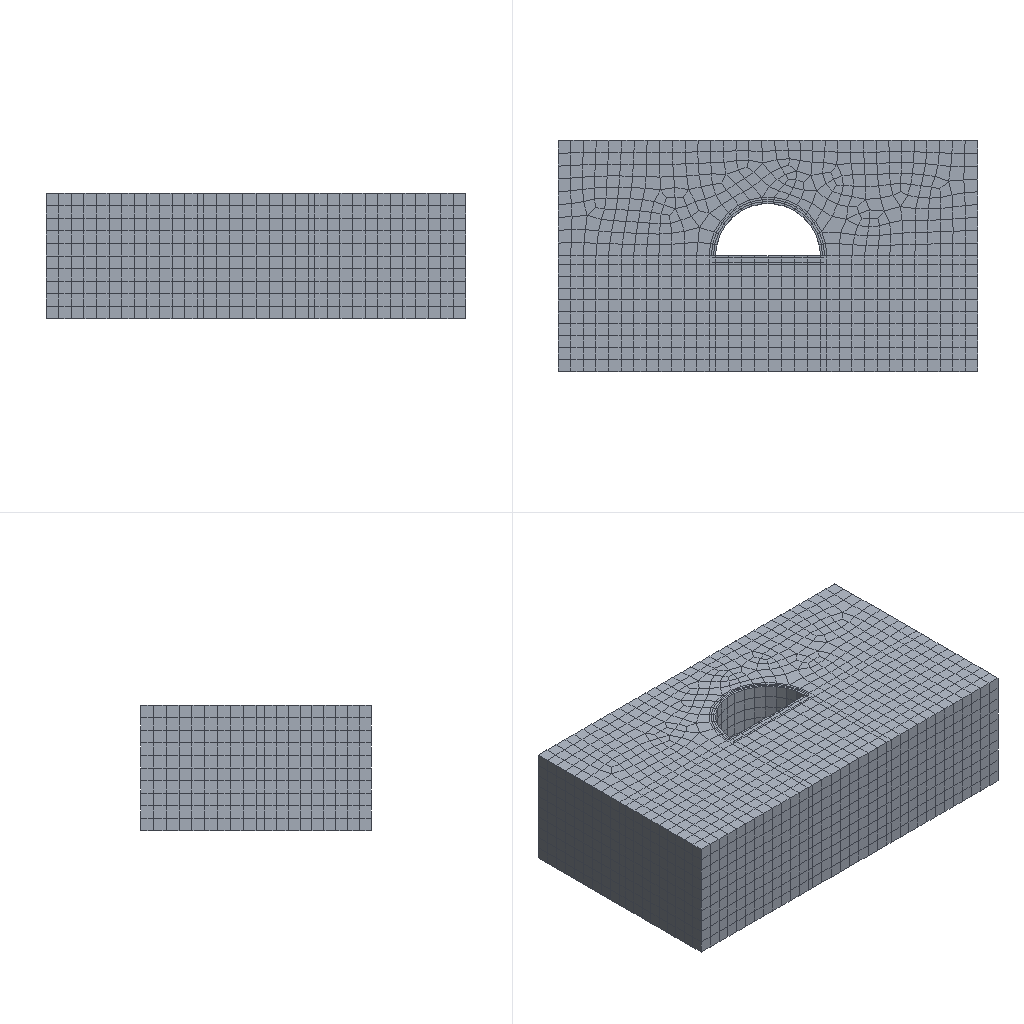Simulation study | abaqus
Set-up summary:
category,name,step,type,value,unit,region
solver,abaqus
solver,version,,,Abaqus/Standard 2020
units,not stated in the deck,,not stated
analysis,deck,,static,static
load_step,Step-1,Step-1,static
load_step,requested,,,1
mesh,nodes,,,8613
mesh,elements,,,7150
element_type,S4R,,shell,460
element_type,C3D8,,solid,6690
load,load commands in deck,,count,2
bc,support commands in deck,,count,7
material,CONCRETE,,in results
material,REBAR,,in results
material,SOIL,,in results
check,setup vs results,,match,"per instance, exact: element labels, types and connectivity; labels of the nodes the elements use; coordinates of those nodes at SINGLE_PRECISION in 5 of 5 instance(s)"
Abaqus input file, long lists of numbers shortened:
*Heading
** Job name: Job-1 Model name: Model-1
** Generated by: Abaqus/CAE 2020
*Preprint, echo=NO, model=NO, history=NO, contact=NO
**
** PARTS
**
*Part, name=Part-1
*Node
      1,  -2.8,   1.1,           6.
      2,  -2.8,   1.1,           0.
** (8061 more lines like these left out)
*Element, type=C3D8
  1,  98, 643, 742,  77,   1,  41,  58,   4
  2, 643, 644, 743, 742,  41,  42,  57,  58
** (6688 more lines like these left out)
*Nset, nset=Set-1
    1,    2,    3,    4,    5,    6,    7,    8,    9,   10,   13,   14,   15,   16,   17,   18
   19,   20,   21,   22,   25,   26,   27,   28,   29,   30,   31,   32,   33,   34,   35,   36
** (487 more lines like these left out)
*Elset, elset=Set-1
    1,    2,    3,    4,    5,    6,    7,    8,    9,   10,   11,   12,   13,   14,   15,   16
   17,   18,   19,   20,   21,   22,   23,   24,   25,   26,   27,   28,   29,   30,   31,   32
** (401 more lines like these left out)
*Nset, nset=Set-2
    1,    2,    3,    4,    9,   10,   11,   12,   20,   21,   23,   24,   25,   26,   27,   28
   41,   42,   43,   44,   45,   46,   47,   48,   49,   50,   51,   52,   53,   54,   55,   56
** (33 more lines like these left out)
*Elset, elset=Set-2
  121,  122,  123,  124,  125,  126,  127,  128,  129,  130, 2021, 2022, 2023, 2024, 2025, 2026
 2027, 2028, 2029, 2030, 2031, 2032, 2033, 2034, 2035, 2036, 2037, 2038, 2039, 2040, 2041, 2042
** (14 more lines like these left out)
*Nset, nset=Set-3
    1,    2,    3,    4,    9,   10,   11,   12,   20,   21,   23,   24,   25,   26,   27,   28
   41,   42,   43,   44,   45,   46,   47,   48,   49,   50,   51,   52,   53,   54,   55,   56
** (33 more lines like these left out)
*Elset, elset=Set-3
  121,  122,  123,  124,  125,  126,  127,  128,  129,  130, 2021, 2022, 2023, 2024, 2025, 2026
 2027, 2028, 2029, 2030, 2031, 2032, 2033, 2034, 2035, 2036, 2037, 2038, 2039, 2040, 2041, 2042
** (14 more lines like these left out)
*Nset, nset=Set-6
    1,    2,    3,    4,    5,    6,    7,    8,    9,   10,   13,   14,   15,   16,   17,   18
   19,   20,   21,   22,   25,   26,   27,   28,   29,   30,   31,   32,   33,   34,   35,   36
** (487 more lines like these left out)
*Elset, elset=Set-6
    1,    2,    3,    4,    5,    6,    7,    8,    9,   10,   11,   12,   13,   14,   15,   16
   17,   18,   19,   20,   21,   22,   23,   24,   25,   26,   27,   28,   29,   30,   31,   32
** (401 more lines like these left out)
*Nset, nset=Set-7
    1,    2,    3,    4,    9,   10,   11,   12,   20,   21,   23,   24,   25,   26,   27,   28
   41,   42,   43,   44,   45,   46,   47,   48,   49,   50,   51,   52,   53,   54,   55,   56
** (33 more lines like these left out)
*Elset, elset=Set-7
  121,  122,  123,  124,  125,  126,  127,  128,  129,  130, 2021, 2022, 2023, 2024, 2025, 2026
 2027, 2028, 2029, 2030, 2031, 2032, 2033, 2034, 2035, 2036, 2037, 2038, 2039, 2040, 2041, 2042
** (14 more lines like these left out)
*Nset, nset=Set-8
    1,    2,    3,    4,    5,    6,    7,    8,    9,   10,   13,   14,   15,   16,   17,   18
   19,   20,   21,   22,   25,   26,   27,   28,   29,   30,   31,   32,   33,   34,   35,   36
** (487 more lines like these left out)
*Elset, elset=Set-8
    1,    2,    3,    4,    5,    6,    7,    8,    9,   10,   11,   12,   13,   14,   15,   16
   17,   18,   19,   20,   21,   22,   23,   24,   25,   26,   27,   28,   29,   30,   31,   32
** (401 more lines like these left out)
*Nset, nset=Set-9
    1,    2,    3,    4,    9,   10,   11,   12,   20,   21,   23,   24,   25,   26,   27,   28
   41,   42,   43,   44,   45,   46,   47,   48,   49,   50,   51,   52,   53,   54,   55,   56
** (33 more lines like these left out)
*Elset, elset=Set-9
  121,  122,  123,  124,  125,  126,  127,  128,  129,  130, 2021, 2022, 2023, 2024, 2025, 2026
 2027, 2028, 2029, 2030, 2031, 2032, 2033, 2034, 2035, 2036, 2037, 2038, 2039, 2040, 2041, 2042
** (14 more lines like these left out)
** Section: Section-1-soil
*Solid Section, elset=Set-8, material=soil
,
** Section: Section-2-concrete
*Solid Section, elset=Set-9, material=concrete
,
*End Part
**
*Part, name=rebar-face
*Node
      1,   5.3,           0.,           0.
      2,   4.711,           0.,           0.
** (108 more lines like these left out)
*Element, type=S4R
 1,   1,   2,  12,  11
 2,   2,   3,  13,  12
** (88 more lines like these left out)
*Nset, nset=Set-1, generate
   1,  110,    1
*Elset, elset=Set-1, generate
  1,  90,   1
** Section: rebar
*Shell Section, elset=Set-1, material=rebar
0.001, 5
*End Part
**
*Part, name=rebar2point6
*Node
      1,    2.6,           0.,           6.
      2,   2.535,  0.5786,           6.
** (163 more lines like these left out)
*Element, type=S4R
  1,   1,   2,  17,  16
  2,   2,   3,  18,  17
** (138 more lines like these left out)
*Nset, nset=Set-1, generate
   1,  165,    1
*Elset, elset=Set-1, generate
   1,  140,    1
** Section: rebar
*Shell Section, elset=Set-1, material=rebar
0.001, 5
*End Part
**
*Part, name=rebar2point7
*Node
      1,   2.7,           0.,           6.
      2,   2.632,  0.6008,           6.
** (163 more lines like these left out)
*Element, type=S4R
  1,   1,   2,  17,  16
  2,   2,   3,  18,  17
** (138 more lines like these left out)
*Nset, nset=Set-1, generate
   1,  165,    1
*Elset, elset=Set-1, generate
   1,  140,    1
** Section: rebar
*Shell Section, elset=Set-1, material=rebar
0.001, 5
*End Part
**
**
** ASSEMBLY
**
*Assembly, name=Assembly
**
*Instance, name=Part-1-1, part=Part-1
*End Instance
**
*Instance, name=rebar2point6-1, part=rebar2point6
          0.,          1.5,           0.
*End Instance
**
*Instance, name=rebar2point7-1, part=rebar2point7
          0.,          1.5,           0.
*End Instance
**
*Instance, name=rebar-face-1, part=rebar-face
       -2.65,          1.4,           6.
       -2.65,          1.4,           6., -1.65,          1.4,           6., 90.
*End Instance
**
*Instance, name=rebar-face-1-lin-1-2, part=rebar-face
       -2.65,          1.2,           6.
       -2.65,          1.2,           6., -1.65,          1.2,           6., 90.
*End Instance
**
*Nset, nset=Set-1, instance=Part-1-1
    1,    4,    7,    8,    9,   12,   13,   14,   18,   21,   22,   23,   25,   28,   29,   31
   32,   36,   39,   40,   77,   78,   79,   80,   81,   82,   83,   84,   85,   86,   87,   88
** (44 more lines like these left out)
*Elset, elset=Set-1, instance=Part-1-1
    1,   11,   21,   31,   41,   51,   61,   71,   81,   91,  101,  111,  121,  131,  132,  133
  134,  135,  136,  137,  138,  139,  140,  141,  142,  143,  144,  145,  146,  147,  148,  149
** (40 more lines like these left out)
*Nset, nset=Set-2, instance=Part-1-1
    2,    3,    5,    6,   10,   11,   15,   16,   17,   19,   20,   24,   26,   27,   30,   33
   34,   35,   37,   38,   99,  100,  101,  102,  103,  104,  105,  106,  107,  108,  109,  110
** (44 more lines like these left out)
*Elset, elset=Set-2, instance=Part-1-1
   10,   20,   30,   40,   50,   60,   70,   80,   90,  100,  110,  120,  130, 1103, 1104, 1105
 1106, 1107, 1108, 1109, 1110, 1111, 1112, 1113, 1114, 1115, 1116, 1117, 1118, 1119, 1120, 1121
** (40 more lines like these left out)
*Nset, nset=Set-3, instance=Part-1-1
   31,   32,   33,   34,   35,   36,   38,   39,  364,  365,  366,  367,  368,  369,  370,  371
  372,  373,  374,  375,  376,  377,  378,  379,  380,  381,  382,  383,  384,  385,  386,  387
** (12 more lines like these left out)
*Elset, elset=Set-3, instance=Part-1-1
 3191, 3192, 3193, 3194, 3195, 3196, 3197, 3198, 3199, 3200, 3201, 3202, 3203, 3204, 3205, 3206
 3207, 3208, 3209, 3210, 3211, 3212, 3213, 3214, 3215, 3216, 3217, 3218, 3219, 3220, 3221, 3222
** (10 more lines like these left out)
*Nset, nset=Set-4, instance=Part-1-1
    5,    6,    7,    8,   14,   15,   37,   40,   59,   60,   61,   62,   63,   64,   65,   66
   67,   68,   69,   70,   71,   72,   73,   74,   75,   76,  147,  148,  149,  150,  151,  152
** (12 more lines like these left out)
*Elset, elset=Set-4, instance=Part-1-1
  111,  112,  113,  114,  115,  116,  117,  118,  119,  120,  230,  231,  232,  233,  234,  235
  236,  237,  238,  338,  339,  340,  341,  342,  343,  344,  345,  346,  446,  447,  448,  449
** (10 more lines like these left out)
*Nset, nset=Set-5, instance=Part-1-1
   13,   14,   15,   16,   17,   18,   19,   22,   29,   30,   32,   33,  155,  156,  157,  158
  159,  160,  161,  162,  163,  164,  165,  182,  183,  184,  185,  186,  187,  188,  189,  190
** (23 more lines like these left out)
*Elset, elset=Set-5, instance=Part-1-1
  131,  140,  149,  158,  167,  176,  185,  194,  203,  212,  221,  230,  239,  248,  257,  266
  275,  284,  293,  302,  311,  320,  329,  338,  347,  356,  365,  374,  383,  392,  401,  410
** (20 more lines like these left out)
*Nset, nset=Set-6, instance=Part-1-1
    1,    2,    3,    4,    5,    6,    7,    8,    9,   10,   13,   14,   15,   16,   17,   18
   19,   20,   21,   22,   25,   26,   27,   28,   29,   30,   31,   32,   33,   34,   35,   36
** (487 more lines like these left out)
*Elset, elset=Set-6, instance=Part-1-1
    1,    2,    3,    4,    5,    6,    7,    8,    9,   10,   11,   12,   13,   14,   15,   16
   17,   18,   19,   20,   21,   22,   23,   24,   25,   26,   27,   28,   29,   30,   31,   32
** (401 more lines like these left out)
*Nset, nset=Set-7, instance=Part-1-1, generate
    1,  8063,     1
*Elset, elset=Set-7, instance=Part-1-1, generate
    1,  6690,     1
*Nset, nset=m_Set-8, instance=rebar2point6-1, generate
   1,  165,    1
*Nset, nset=m_Set-8, instance=rebar2point7-1, generate
   1,  165,    1
*Nset, nset=m_Set-8, instance=rebar-face-1, generate
   1,  110,    1
*Nset, nset=m_Set-8, instance=rebar-face-1-lin-1-2, generate
   1,  110,    1
*Elset, elset=m_Set-8, instance=rebar2point6-1, generate
   1,  140,    1
*Elset, elset=m_Set-8, instance=rebar2point7-1, generate
   1,  140,    1
*Elset, elset=m_Set-8, instance=rebar-face-1, generate
  1,  90,   1
*Elset, elset=m_Set-8, instance=rebar-face-1-lin-1-2, generate
  1,  90,   1
*Nset, nset=s_Set-8, instance=Part-1-1, generate
    1,  8063,     1
*Elset, elset=s_Set-8, instance=Part-1-1, generate
    1,  6690,     1
*Elset, elset=_Surf-1_S5, internal, instance=Part-1-1
 3552, 3555, 3562, 3564, 3566, 3573, 3601, 3603, 3610, 3613, 3647, 3648, 3657, 3677, 3683, 3866
 3869, 3876, 3878, 3880, 3887, 3915, 3917, 3924, 3927, 3961, 3962, 3971, 3991, 3997, 4180, 4183
** (8 more lines like these left out)
*Elset, elset=_Surf-1_S3, internal, instance=Part-1-1
 3553, 3554, 3559, 3574, 3575, 3586, 3589, 3591, 3594, 3595, 3596, 3599, 3615, 3636, 3662, 3679
 3715, 3867, 3868, 3873, 3888, 3889, 3900, 3903, 3905, 3908, 3909, 3910, 3913, 3929, 3950, 3976
** (9 more lines like these left out)
*Elset, elset=_Surf-1_S4, internal, instance=Part-1-1, generate
 3582,  6408,   314
*Surface, type=ELEMENT, name=Surf-1
_Surf-1_S5, S5
_Surf-1_S3, S3
_Surf-1_S4, S4
** Constraint: Constraint-1
*Embedded Element, host elset=s_Set-8
m_Set-8
*End Assembly
*Amplitude, name=Amp-1
             0.,              0.,              1.,              1.
**
** MATERIALS
**
*Material, name=concrete
*Density
2500.,
*Elastic
 2.5e+10, 0.2
*Material, name=rebar
*Density
7860.,
*Elastic
 2.1e+11, 0.3
*Material, name=soil
*Density
1800.,
*Elastic
 4.79e+07, 0.35
*Mohr Coulomb
25.,0.
*Mohr Coulomb Hardening
25000.,0.
**
** BOUNDARY CONDITIONS
**
** Name: BC-1 Type: 位移/转角
*Boundary
Set-1, 3, 3
** Name: BC-2 Type: 位移/转角
*Boundary
Set-2, 3, 3
** Name: BC-3 Type: 位移/转角
*Boundary
Set-3, 1, 1
** Name: BC-4 Type: 位移/转角
*Boundary
Set-4, 1, 1
** Name: BC-5 Type: 位移/转角
*Boundary
Set-5, 1, 1
Set-5, 2, 2
Set-5, 3, 3
**
** PREDEFINED FIELDS
**
** Name: Predefined Field-1   Type: Geostatic stress
*Initial Conditions, type=STRESS, GEOSTATIC
Set-6, 0., 6., -20000., -4., 2., 2.
** ----------------------------------------------------------------
**
** STEP: Step-1
**
*Step, name=Step-1, nlgeom=YES, inc=1000
*Static, stabilize=0.0002, allsdtol=0.05, continue=NO
0.01, 1., 1e-05, 1.
**
** LOADS
**
** Name: Load-2   Type: Pressure
*Dsload, amplitude=Amp-1
Surf-1, P, 1e+06
** Name: Load-3   Type: Gravity
*Dload
, GRAV, 9.8, 0., -1., 0.
**
** OUTPUT REQUESTS
**
*Restart, write, frequency=0
**
** FIELD OUTPUT: F-Output-1
**
*Output, field
*Node Output
CF, RF, RM, RT, TF, U, V
*Element Output, directions=YES
E, LE, MISES, MISESMAX, PE, PEEQ, PEMAG, S, SF, SSAVG
*Contact Output
CDISP, CSTRESS
**
** HISTORY OUTPUT: H-Output-1
**
*Output, history, variable=PRESELECT
*End Step
Results summary:
result,step,,completed,increments=11 time=1.0/1.0
result,analysis,,,static
result,last_loadstep,,,1
result,primary field,,,"U, UR"
result,reaction total,,FX,41.519,model units
result,reaction total,,FY,142407566.555,model units
result,reaction total,,FZ,18885.436,model units